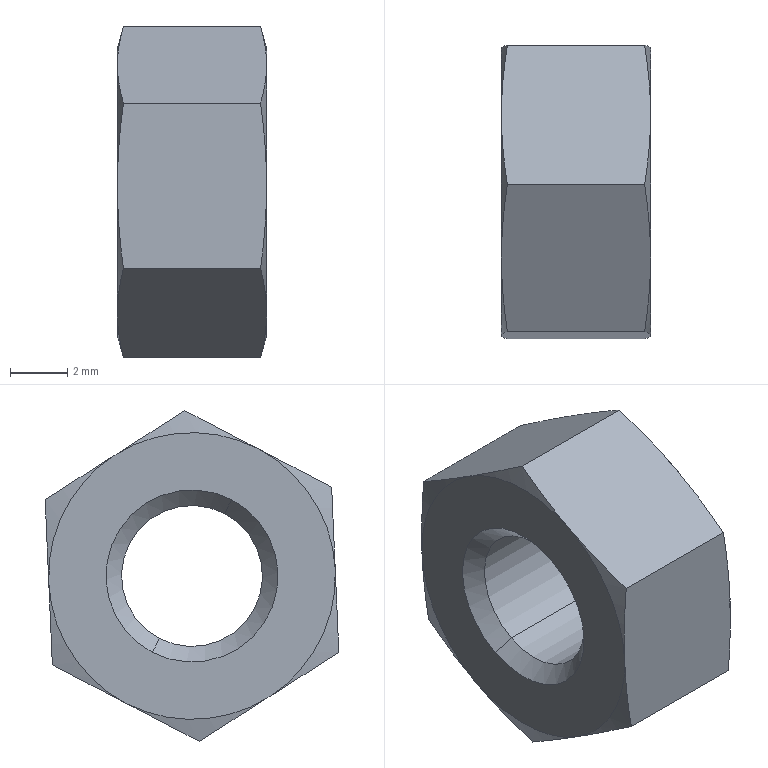Part | NX | features 2 2 | 1 solid | 26 faces | box 5.2 x 10.241 x 11.536 mm | volume 345.697 mm3 | cone 16 | plane 8 | cylinder 2 | commonest cylinder face diameters 4.917 x2
STEP:
#1=CARTESIAN_POINT('',(-91.959,96.265,-644.397));
#2=VERTEX_POINT('',#1);
#3=CARTESIAN_POINT('',(-91.959,93.994,-640.036));
#4=VERTEX_POINT('',#3);
#5=CARTESIAN_POINT('',(-91.959,95.129,-642.216));
#6=DIRECTION('',(1.,0.,0.));
#7=DIRECTION('',(0.,-0.4619,0.8869));
#8=AXIS2_PLACEMENT_3D('',#5,#6,#7);
#9=CIRCLE('',#8,2.458);
#10=EDGE_CURVE('',#2,#4,#9,.T.);
#11=ORIENTED_EDGE('',*,*,#10,.F.);
#12=CARTESIAN_POINT('',(-87.842,96.265,-644.397));
#13=VERTEX_POINT('',#12);
#14=CARTESIAN_POINT('',(-89.9,96.265,-644.397));
#15=DIRECTION('',(1.,0.,0.));
#16=VECTOR('',#15,1000.);
#17=LINE('',#14,#16);
#18=EDGE_CURVE('',#2,#13,#17,.T.);
#19=ORIENTED_EDGE('',*,*,#18,.T.);
#20=CARTESIAN_POINT('',(-87.842,93.994,-640.036));
#21=VERTEX_POINT('',#20);
#22=CARTESIAN_POINT('',(-87.842,95.129,-642.216));
#23=DIRECTION('',(-1.,0.,0.));
#24=DIRECTION('',(0.,-0.4619,0.8869));
#25=AXIS2_PLACEMENT_3D('',#22,#23,#24);
#26=CIRCLE('',#25,2.458);
#27=EDGE_CURVE('',#21,#13,#26,.T.);
#28=ORIENTED_EDGE('',*,*,#27,.F.);
#29=CARTESIAN_POINT('',(-89.9,93.994,-640.036));
#30=DIRECTION('',(1.,0.,0.));
#31=VECTOR('',#30,1000.);
#32=LINE('',#29,#31);
#33=EDGE_CURVE('',#21,#4,#32,.F.);
#34=ORIENTED_EDGE('',*,*,#33,.T.);
#35=EDGE_LOOP('',(#11,#19,#28,#34));
#36=FACE_BOUND('',#35,.T.);
#37=CARTESIAN_POINT('',(-89.9,95.129,-642.216));
#38=DIRECTION('',(1.,0.,0.));
#39=DIRECTION('',(0.,0.4619,-0.8869));
#40=AXIS2_PLACEMENT_3D('',#37,#38,#39);
#41=CYLINDRICAL_SURFACE('',#40,2.458);
#42=ADVANCED_FACE('',(#36),#41,.F.);
#43=ORIENTED_EDGE('',*,*,#10,.T.);
#44=CARTESIAN_POINT('',(-92.5,93.744,-639.556));
#45=VERTEX_POINT('',#44);
#46=CARTESIAN_POINT('',(-92.5,93.744,-639.556));
#47=DIRECTION('',(-0.7071,-0.3266,0.6272));
#48=VECTOR('',#47,1000.);
#49=LINE('',#46,#48);
#50=EDGE_CURVE('',#45,#4,#49,.F.);
#51=ORIENTED_EDGE('',*,*,#50,.F.);
#52=CARTESIAN_POINT('',(-92.5,96.515,-644.877));
#53=VERTEX_POINT('',#52);
#54=CARTESIAN_POINT('',(-92.5,95.129,-642.216));
#55=DIRECTION('',(1.,0.,0.));
#56=DIRECTION('',(0.,0.4619,-0.8869));
#57=AXIS2_PLACEMENT_3D('',#54,#55,#56);
#58=CIRCLE('',#57,3.);
#59=EDGE_CURVE('',#53,#45,#58,.T.);
#60=ORIENTED_EDGE('',*,*,#59,.F.);
#61=CARTESIAN_POINT('',(-92.5,96.515,-644.877));
#62=DIRECTION('',(-0.7071,0.3266,-0.6272));
#63=VECTOR('',#62,1000.);
#64=LINE('',#61,#63);
#65=EDGE_CURVE('',#2,#53,#64,.T.);
#66=ORIENTED_EDGE('',*,*,#65,.F.);
#67=EDGE_LOOP('',(#43,#51,#60,#66));
#68=FACE_BOUND('',#67,.T.);
#69=CARTESIAN_POINT('',(-92.5,95.129,-642.216));
#70=DIRECTION('',(-1.,0.,0.));
#71=DIRECTION('',(0.,-0.4619,0.8869));
#72=AXIS2_PLACEMENT_3D('',#69,#70,#71);
#73=CONICAL_SURFACE('',#72,3.,0.7854);
#74=ADVANCED_FACE('',(#68),#73,.F.);
#75=ORIENTED_EDGE('',*,*,#27,.T.);
#76=CARTESIAN_POINT('',(-87.3,96.515,-644.877));
#77=VERTEX_POINT('',#76);
#78=CARTESIAN_POINT('',(-87.3,96.515,-644.877));
#79=DIRECTION('',(0.7071,0.3266,-0.6272));
#80=VECTOR('',#79,1000.);
#81=LINE('',#78,#80);
#82=EDGE_CURVE('',#77,#13,#81,.F.);
#83=ORIENTED_EDGE('',*,*,#82,.F.);
#84=CARTESIAN_POINT('',(-87.3,93.744,-639.556));
#85=VERTEX_POINT('',#84);
#86=CARTESIAN_POINT('',(-87.3,95.129,-642.216));
#87=DIRECTION('',(-1.,0.,0.));
#88=DIRECTION('',(0.,-0.4619,0.8869));
#89=AXIS2_PLACEMENT_3D('',#86,#87,#88);
#90=CIRCLE('',#89,3.);
#91=EDGE_CURVE('',#85,#77,#90,.T.);
#92=ORIENTED_EDGE('',*,*,#91,.F.);
#93=CARTESIAN_POINT('',(-87.3,93.744,-639.556));
#94=DIRECTION('',(0.7071,-0.3266,0.6272));
#95=VECTOR('',#94,1000.);
#96=LINE('',#93,#95);
#97=EDGE_CURVE('',#21,#85,#96,.T.);
#98=ORIENTED_EDGE('',*,*,#97,.F.);
#99=EDGE_LOOP('',(#75,#83,#92,#98));
#100=FACE_BOUND('',#99,.T.);
#101=CARTESIAN_POINT('',(-87.3,95.129,-642.216));
#102=DIRECTION('',(1.,0.,0.));
#103=DIRECTION('',(0.,0.4619,-0.8869));
#104=AXIS2_PLACEMENT_3D('',#101,#102,#103);
#105=CONICAL_SURFACE('',#104,3.,0.7854);
#106=ADVANCED_FACE('',(#100),#105,.F.);
#107=ORIENTED_EDGE('',*,*,#18,.F.);
#108=CARTESIAN_POINT('',(-91.959,95.129,-642.216));
#109=DIRECTION('',(1.,0.,0.));
#110=DIRECTION('',(0.,-0.4619,0.8869));
#111=AXIS2_PLACEMENT_3D('',#108,#109,#110);
#112=CIRCLE('',#111,2.458);
#113=EDGE_CURVE('',#4,#2,#112,.T.);
#114=ORIENTED_EDGE('',*,*,#113,.F.);
#115=ORIENTED_EDGE('',*,*,#33,.F.);
#116=CARTESIAN_POINT('',(-87.842,95.129,-642.216));
#117=DIRECTION('',(-1.,0.,0.));
#118=DIRECTION('',(0.,-0.4619,0.8869));
#119=AXIS2_PLACEMENT_3D('',#116,#117,#118);
#120=CIRCLE('',#119,2.458);
#121=EDGE_CURVE('',#13,#21,#120,.T.);
#122=ORIENTED_EDGE('',*,*,#121,.F.);
#123=EDGE_LOOP('',(#107,#114,#115,#122));
#124=FACE_BOUND('',#123,.T.);
#125=CARTESIAN_POINT('',(-89.9,95.129,-642.216));
#126=DIRECTION('',(1.,0.,0.));
#127=DIRECTION('',(0.,0.4619,-0.8869));
#128=AXIS2_PLACEMENT_3D('',#125,#126,#127);
#129=CYLINDRICAL_SURFACE('',#128,2.458);
#130=ADVANCED_FACE('',(#124),#129,.F.);
#131=ORIENTED_EDGE('',*,*,#50,.T.);
#132=ORIENTED_EDGE('',*,*,#113,.T.);
#133=ORIENTED_EDGE('',*,*,#65,.T.);
#134=CARTESIAN_POINT('',(-92.5,95.129,-642.216));
#135=DIRECTION('',(1.,0.,0.));
#136=DIRECTION('',(0.,0.4619,-0.8869));
#137=AXIS2_PLACEMENT_3D('',#134,#135,#136);
#138=CIRCLE('',#137,3.);
#139=EDGE_CURVE('',#45,#53,#138,.T.);
#140=ORIENTED_EDGE('',*,*,#139,.F.);
#141=EDGE_LOOP('',(#131,#132,#133,#140));
#142=FACE_BOUND('',#141,.T.);
#143=CARTESIAN_POINT('',(-92.5,95.129,-642.216));
#144=DIRECTION('',(-1.,0.,0.));
#145=DIRECTION('',(0.,-0.4619,0.8869));
#146=AXIS2_PLACEMENT_3D('',#143,#144,#145);
#147=CONICAL_SURFACE('',#146,3.,0.7854);
#148=ADVANCED_FACE('',(#142),#147,.F.);
#149=ORIENTED_EDGE('',*,*,#82,.T.);
#150=ORIENTED_EDGE('',*,*,#121,.T.);
#151=ORIENTED_EDGE('',*,*,#97,.T.);
#152=CARTESIAN_POINT('',(-87.3,95.129,-642.216));
#153=DIRECTION('',(-1.,0.,0.));
#154=DIRECTION('',(0.,-0.4619,0.8869));
#155=AXIS2_PLACEMENT_3D('',#152,#153,#154);
#156=CIRCLE('',#155,3.);
#157=EDGE_CURVE('',#77,#85,#156,.T.);
#158=ORIENTED_EDGE('',*,*,#157,.F.);
#159=EDGE_LOOP('',(#149,#150,#151,#158));
#160=FACE_BOUND('',#159,.T.);
#161=CARTESIAN_POINT('',(-87.3,95.129,-642.216));
#162=DIRECTION('',(1.,0.,0.));
#163=DIRECTION('',(0.,0.4619,-0.8869));
#164=AXIS2_PLACEMENT_3D('',#161,#162,#163);
#165=CONICAL_SURFACE('',#164,3.,0.7854);
#166=ADVANCED_FACE('',(#160),#165,.F.);
#167=ORIENTED_EDGE('',*,*,#59,.T.);
#168=ORIENTED_EDGE('',*,*,#139,.T.);
#169=EDGE_LOOP('',(#167,#168));
#170=FACE_BOUND('',#169,.T.);
#171=CARTESIAN_POINT('',(-92.5,90.134,-641.999));
#172=VERTEX_POINT('',#171);
#173=CARTESIAN_POINT('',(-92.5,92.82,-637.782));
#174=VERTEX_POINT('',#173);
#175=CARTESIAN_POINT('',(-92.5,95.129,-642.216));
#176=DIRECTION('',(-1.,0.,0.));
#177=DIRECTION('',(0.,-0.4619,0.8869));
#178=AXIS2_PLACEMENT_3D('',#175,#176,#177);
#179=CIRCLE('',#178,5.);
#180=EDGE_CURVE('',#172,#174,#179,.T.);
#181=ORIENTED_EDGE('',*,*,#180,.T.);
#182=CARTESIAN_POINT('',(-92.5,97.815,-637.999));
#183=VERTEX_POINT('',#182);
#184=CARTESIAN_POINT('',(-92.5,95.129,-642.216));
#185=DIRECTION('',(-1.,0.,0.));
#186=DIRECTION('',(0.,-0.4619,0.8869));
#187=AXIS2_PLACEMENT_3D('',#184,#185,#186);
#188=CIRCLE('',#187,5.);
#189=EDGE_CURVE('',#174,#183,#188,.T.);
#190=ORIENTED_EDGE('',*,*,#189,.T.);
#191=CARTESIAN_POINT('',(-92.5,100.125,-642.434));
#192=VERTEX_POINT('',#191);
#193=CARTESIAN_POINT('',(-92.5,95.129,-642.216));
#194=DIRECTION('',(-1.,0.,0.));
#195=DIRECTION('',(0.,-0.4619,0.8869));
#196=AXIS2_PLACEMENT_3D('',#193,#194,#195);
#197=CIRCLE('',#196,5.);
#198=EDGE_CURVE('',#183,#192,#197,.T.);
#199=ORIENTED_EDGE('',*,*,#198,.T.);
#200=CARTESIAN_POINT('',(-92.5,97.439,-646.651));
#201=VERTEX_POINT('',#200);
#202=CARTESIAN_POINT('',(-92.5,95.129,-642.216));
#203=DIRECTION('',(-1.,0.,0.));
#204=DIRECTION('',(0.,-0.4619,0.8869));
#205=AXIS2_PLACEMENT_3D('',#202,#203,#204);
#206=CIRCLE('',#205,5.);
#207=EDGE_CURVE('',#192,#201,#206,.T.);
#208=ORIENTED_EDGE('',*,*,#207,.T.);
#209=CARTESIAN_POINT('',(-92.5,92.444,-646.434));
#210=VERTEX_POINT('',#209);
#211=CARTESIAN_POINT('',(-92.5,95.129,-642.216));
#212=DIRECTION('',(-1.,0.,0.));
#213=DIRECTION('',(0.,-0.4619,0.8869));
#214=AXIS2_PLACEMENT_3D('',#211,#212,#213);
#215=CIRCLE('',#214,5.);
#216=EDGE_CURVE('',#201,#210,#215,.T.);
#217=ORIENTED_EDGE('',*,*,#216,.T.);
#218=CARTESIAN_POINT('',(-92.5,95.129,-642.216));
#219=DIRECTION('',(-1.,0.,0.));
#220=DIRECTION('',(0.,-0.4619,0.8869));
#221=AXIS2_PLACEMENT_3D('',#218,#219,#220);
#222=CIRCLE('',#221,5.);
#223=EDGE_CURVE('',#210,#172,#222,.T.);
#224=ORIENTED_EDGE('',*,*,#223,.T.);
#225=EDGE_LOOP('',(#181,#190,#199,#208,#217,#224));
#226=FACE_BOUND('',#225,.T.);
#227=CARTESIAN_POINT('',(-92.5,97.347,-641.062));
#228=DIRECTION('',(-1.,0.,0.));
#229=DIRECTION('',(0.,-0.4619,0.8869));
#230=AXIS2_PLACEMENT_3D('',#227,#228,#229);
#231=PLANE('',#230);
#232=ADVANCED_FACE('',(#170,#226),#231,.T.);
#233=ORIENTED_EDGE('',*,*,#91,.T.);
#234=ORIENTED_EDGE('',*,*,#157,.T.);
#235=EDGE_LOOP('',(#233,#234));
#236=FACE_BOUND('',#235,.T.);
#237=CARTESIAN_POINT('',(-87.3,92.444,-646.434));
#238=VERTEX_POINT('',#237);
#239=CARTESIAN_POINT('',(-87.3,97.439,-646.651));
#240=VERTEX_POINT('',#239);
#241=CARTESIAN_POINT('',(-87.3,95.129,-642.216));
#242=DIRECTION('',(1.,0.,0.));
#243=DIRECTION('',(0.,0.4619,-0.8869));
#244=AXIS2_PLACEMENT_3D('',#241,#242,#243);
#245=CIRCLE('',#244,5.);
#246=EDGE_CURVE('',#238,#240,#245,.T.);
#247=ORIENTED_EDGE('',*,*,#246,.T.);
#248=CARTESIAN_POINT('',(-87.3,100.125,-642.434));
#249=VERTEX_POINT('',#248);
#250=CARTESIAN_POINT('',(-87.3,95.129,-642.216));
#251=DIRECTION('',(1.,0.,0.));
#252=DIRECTION('',(0.,0.4619,-0.8869));
#253=AXIS2_PLACEMENT_3D('',#250,#251,#252);
#254=CIRCLE('',#253,5.);
#255=EDGE_CURVE('',#240,#249,#254,.T.);
#256=ORIENTED_EDGE('',*,*,#255,.T.);
#257=CARTESIAN_POINT('',(-87.3,97.815,-637.999));
#258=VERTEX_POINT('',#257);
#259=CARTESIAN_POINT('',(-87.3,95.129,-642.216));
#260=DIRECTION('',(1.,0.,0.));
#261=DIRECTION('',(0.,0.4619,-0.8869));
#262=AXIS2_PLACEMENT_3D('',#259,#260,#261);
#263=CIRCLE('',#262,5.);
#264=EDGE_CURVE('',#249,#258,#263,.T.);
#265=ORIENTED_EDGE('',*,*,#264,.T.);
#266=CARTESIAN_POINT('',(-87.3,92.82,-637.782));
#267=VERTEX_POINT('',#266);
#268=CARTESIAN_POINT('',(-87.3,95.129,-642.216));
#269=DIRECTION('',(1.,0.,0.));
#270=DIRECTION('',(0.,0.4619,-0.8869));
#271=AXIS2_PLACEMENT_3D('',#268,#269,#270);
#272=CIRCLE('',#271,5.);
#273=EDGE_CURVE('',#258,#267,#272,.T.);
#274=ORIENTED_EDGE('',*,*,#273,.T.);
#275=CARTESIAN_POINT('',(-87.3,90.134,-641.999));
#276=VERTEX_POINT('',#275);
#277=CARTESIAN_POINT('',(-87.3,95.129,-642.216));
#278=DIRECTION('',(1.,0.,0.));
#279=DIRECTION('',(0.,0.4619,-0.8869));
#280=AXIS2_PLACEMENT_3D('',#277,#278,#279);
#281=CIRCLE('',#280,5.);
#282=EDGE_CURVE('',#267,#276,#281,.T.);
#283=ORIENTED_EDGE('',*,*,#282,.T.);
#284=CARTESIAN_POINT('',(-87.3,95.129,-642.216));
#285=DIRECTION('',(1.,0.,0.));
#286=DIRECTION('',(0.,0.4619,-0.8869));
#287=AXIS2_PLACEMENT_3D('',#284,#285,#286);
#288=CIRCLE('',#287,5.);
#289=EDGE_CURVE('',#276,#238,#288,.T.);
#290=ORIENTED_EDGE('',*,*,#289,.T.);
#291=EDGE_LOOP('',(#247,#256,#265,#274,#283,#290));
#292=FACE_BOUND('',#291,.T.);
#293=CARTESIAN_POINT('',(-87.3,97.347,-641.062));
#294=DIRECTION('',(1.,0.,0.));
#295=DIRECTION('',(0.,0.4619,-0.8869));
#296=AXIS2_PLACEMENT_3D('',#293,#294,#295);
#297=PLANE('',#296);
#298=ADVANCED_FACE('',(#236,#292),#297,.T.);
#299=CARTESIAN_POINT('',(-92.293,95.38,-636.448));
#300=VERTEX_POINT('',#299);
#301=CARTESIAN_POINT('',(-92.293,95.38,-636.448));
#302=CARTESIAN_POINT('',(-92.421,96.188,-636.963));
#303=CARTESIAN_POINT('',(-92.5,96.999,-637.479));
#304=CARTESIAN_POINT('',(-92.5,97.815,-637.999));
#305=B_SPLINE_CURVE_WITH_KNOTS('',3,(#301,#302,#303,#304),.UNSPECIFIED.,.F.,.F.,(4,4),(0.,0.002894),.UNSPECIFIED.);
#306=EDGE_CURVE('',#300,#183,#305,.T.);
#307=ORIENTED_EDGE('',*,*,#306,.T.);
#308=ORIENTED_EDGE('',*,*,#189,.F.);
#309=CARTESIAN_POINT('',(-92.5,92.82,-637.782));
#310=CARTESIAN_POINT('',(-92.5,93.678,-637.335));
#311=CARTESIAN_POINT('',(-92.421,94.531,-636.891));
#312=CARTESIAN_POINT('',(-92.293,95.38,-636.448));
#313=B_SPLINE_CURVE_WITH_KNOTS('',3,(#309,#310,#311,#312),.UNSPECIFIED.,.F.,.F.,(4,4),(0.,0.002894),.UNSPECIFIED.);
#314=EDGE_CURVE('',#174,#300,#313,.T.);
#315=ORIENTED_EDGE('',*,*,#314,.T.);
#316=EDGE_LOOP('',(#307,#308,#315));
#317=FACE_BOUND('',#316,.T.);
#318=CARTESIAN_POINT('',(-92.291,95.129,-642.216));
#319=DIRECTION('',(1.,0.,0.));
#320=DIRECTION('',(0.,0.4619,-0.8869));
#321=AXIS2_PLACEMENT_3D('',#318,#319,#320);
#322=CONICAL_SURFACE('',#321,5.778,1.309);
#323=ADVANCED_FACE('',(#317),#322,.T.);
#324=CARTESIAN_POINT('',(-92.293,90.26,-639.115));
#325=VERTEX_POINT('',#324);
#326=CARTESIAN_POINT('',(-92.293,90.26,-639.115));
#327=CARTESIAN_POINT('',(-92.421,91.109,-638.673));
#328=CARTESIAN_POINT('',(-92.5,91.962,-638.229));
#329=CARTESIAN_POINT('',(-92.5,92.82,-637.782));
#330=B_SPLINE_CURVE_WITH_KNOTS('',3,(#326,#327,#328,#329),.UNSPECIFIED.,.F.,.F.,(4,4),(0.,0.002894),.UNSPECIFIED.);
#331=EDGE_CURVE('',#325,#174,#330,.T.);
#332=ORIENTED_EDGE('',*,*,#331,.T.);
#333=ORIENTED_EDGE('',*,*,#180,.F.);
#334=CARTESIAN_POINT('',(-92.5,90.134,-641.999));
#335=CARTESIAN_POINT('',(-92.5,90.176,-641.033));
#336=CARTESIAN_POINT('',(-92.421,90.218,-640.072));
#337=CARTESIAN_POINT('',(-92.293,90.26,-639.115));
#338=B_SPLINE_CURVE_WITH_KNOTS('',3,(#334,#335,#336,#337),.UNSPECIFIED.,.F.,.F.,(4,4),(0.,0.002894),.UNSPECIFIED.);
#339=EDGE_CURVE('',#172,#325,#338,.T.);
#340=ORIENTED_EDGE('',*,*,#339,.T.);
#341=EDGE_LOOP('',(#332,#333,#340));
#342=FACE_BOUND('',#341,.T.);
#343=CARTESIAN_POINT('',(-92.291,95.129,-642.216));
#344=DIRECTION('',(1.,0.,0.));
#345=DIRECTION('',(0.,0.4619,-0.8869));
#346=AXIS2_PLACEMENT_3D('',#343,#344,#345);
#347=CONICAL_SURFACE('',#346,5.778,1.309);
#348=ADVANCED_FACE('',(#342),#347,.T.);
#349=CARTESIAN_POINT('',(-92.293,90.009,-644.883));
#350=VERTEX_POINT('',#349);
#351=CARTESIAN_POINT('',(-92.5,92.444,-646.434));
#352=CARTESIAN_POINT('',(-92.5,91.628,-645.914));
#353=CARTESIAN_POINT('',(-92.421,90.817,-645.398));
#354=CARTESIAN_POINT('',(-92.293,90.009,-644.883));
#355=B_SPLINE_CURVE_WITH_KNOTS('',3,(#351,#352,#353,#354),.UNSPECIFIED.,.F.,.F.,(4,4),(0.,0.002894),.UNSPECIFIED.);
#356=EDGE_CURVE('',#210,#350,#355,.T.);
#357=ORIENTED_EDGE('',*,*,#356,.T.);
#358=CARTESIAN_POINT('',(-92.293,90.009,-644.883));
#359=CARTESIAN_POINT('',(-92.421,90.05,-643.926));
#360=CARTESIAN_POINT('',(-92.5,90.092,-642.966));
#361=CARTESIAN_POINT('',(-92.5,90.134,-641.999));
#362=B_SPLINE_CURVE_WITH_KNOTS('',3,(#358,#359,#360,#361),.UNSPECIFIED.,.F.,.F.,(4,4),(0.,0.002894),.UNSPECIFIED.);
#363=EDGE_CURVE('',#350,#172,#362,.T.);
#364=ORIENTED_EDGE('',*,*,#363,.T.);
#365=ORIENTED_EDGE('',*,*,#223,.F.);
#366=EDGE_LOOP('',(#357,#364,#365));
#367=FACE_BOUND('',#366,.T.);
#368=CARTESIAN_POINT('',(-92.291,95.129,-642.216));
#369=DIRECTION('',(1.,0.,0.));
#370=DIRECTION('',(0.,0.4619,-0.8869));
#371=AXIS2_PLACEMENT_3D('',#368,#369,#370);
#372=CONICAL_SURFACE('',#371,5.778,1.309);
#373=ADVANCED_FACE('',(#367),#372,.T.);
#374=ORIENTED_EDGE('',*,*,#216,.F.);
#375=CARTESIAN_POINT('',(-92.293,94.879,-647.984));
#376=VERTEX_POINT('',#375);
#377=CARTESIAN_POINT('',(-92.5,97.439,-646.651));
#378=CARTESIAN_POINT('',(-92.5,96.581,-647.098));
#379=CARTESIAN_POINT('',(-92.421,95.728,-647.542));
#380=CARTESIAN_POINT('',(-92.293,94.879,-647.984));
#381=B_SPLINE_CURVE_WITH_KNOTS('',3,(#377,#378,#379,#380),.UNSPECIFIED.,.F.,.F.,(4,4),(0.,0.002894),.UNSPECIFIED.);
#382=EDGE_CURVE('',#201,#376,#381,.T.);
#383=ORIENTED_EDGE('',*,*,#382,.T.);
#384=CARTESIAN_POINT('',(-92.293,94.879,-647.984));
#385=CARTESIAN_POINT('',(-92.421,94.071,-647.47));
#386=CARTESIAN_POINT('',(-92.5,93.259,-646.953));
#387=CARTESIAN_POINT('',(-92.5,92.444,-646.434));
#388=B_SPLINE_CURVE_WITH_KNOTS('',3,(#384,#385,#386,#387),.UNSPECIFIED.,.F.,.F.,(4,4),(0.,0.002894),.UNSPECIFIED.);
#389=EDGE_CURVE('',#376,#210,#388,.T.);
#390=ORIENTED_EDGE('',*,*,#389,.T.);
#391=EDGE_LOOP('',(#374,#383,#390));
#392=FACE_BOUND('',#391,.T.);
#393=CARTESIAN_POINT('',(-92.291,95.129,-642.216));
#394=DIRECTION('',(1.,0.,0.));
#395=DIRECTION('',(0.,0.4619,-0.8869));
#396=AXIS2_PLACEMENT_3D('',#393,#394,#395);
#397=CONICAL_SURFACE('',#396,5.778,1.309);
#398=ADVANCED_FACE('',(#392),#397,.T.);
#399=ORIENTED_EDGE('',*,*,#207,.F.);
#400=CARTESIAN_POINT('',(-92.293,99.999,-645.318));
#401=VERTEX_POINT('',#400);
#402=CARTESIAN_POINT('',(-92.5,100.125,-642.434));
#403=CARTESIAN_POINT('',(-92.5,100.083,-643.4));
#404=CARTESIAN_POINT('',(-92.421,100.041,-644.361));
#405=CARTESIAN_POINT('',(-92.293,99.999,-645.318));
#406=B_SPLINE_CURVE_WITH_KNOTS('',3,(#402,#403,#404,#405),.UNSPECIFIED.,.F.,.F.,(4,4),(0.,0.002894),.UNSPECIFIED.);
#407=EDGE_CURVE('',#192,#401,#406,.T.);
#408=ORIENTED_EDGE('',*,*,#407,.T.);
#409=CARTESIAN_POINT('',(-92.293,99.999,-645.318));
#410=CARTESIAN_POINT('',(-92.421,99.15,-645.76));
#411=CARTESIAN_POINT('',(-92.5,98.297,-646.204));
#412=CARTESIAN_POINT('',(-92.5,97.439,-646.651));
#413=B_SPLINE_CURVE_WITH_KNOTS('',3,(#409,#410,#411,#412),.UNSPECIFIED.,.F.,.F.,(4,4),(0.,0.002894),.UNSPECIFIED.);
#414=EDGE_CURVE('',#401,#201,#413,.T.);
#415=ORIENTED_EDGE('',*,*,#414,.T.);
#416=EDGE_LOOP('',(#399,#408,#415));
#417=FACE_BOUND('',#416,.T.);
#418=CARTESIAN_POINT('',(-92.291,95.129,-642.216));
#419=DIRECTION('',(1.,0.,0.));
#420=DIRECTION('',(0.,0.4619,-0.8869));
#421=AXIS2_PLACEMENT_3D('',#418,#419,#420);
#422=CONICAL_SURFACE('',#421,5.778,1.309);
#423=ADVANCED_FACE('',(#417),#422,.T.);
#424=ORIENTED_EDGE('',*,*,#198,.F.);
#425=CARTESIAN_POINT('',(-92.293,100.25,-639.55));
#426=VERTEX_POINT('',#425);
#427=CARTESIAN_POINT('',(-92.5,97.815,-637.999));
#428=CARTESIAN_POINT('',(-92.5,98.631,-638.519));
#429=CARTESIAN_POINT('',(-92.421,99.442,-639.035));
#430=CARTESIAN_POINT('',(-92.293,100.25,-639.55));
#431=B_SPLINE_CURVE_WITH_KNOTS('',3,(#427,#428,#429,#430),.UNSPECIFIED.,.F.,.F.,(4,4),(0.,0.002894),.UNSPECIFIED.);
#432=EDGE_CURVE('',#183,#426,#431,.T.);
#433=ORIENTED_EDGE('',*,*,#432,.T.);
#434=CARTESIAN_POINT('',(-92.293,100.25,-639.55));
#435=CARTESIAN_POINT('',(-92.421,100.208,-640.507));
#436=CARTESIAN_POINT('',(-92.5,100.167,-641.467));
#437=CARTESIAN_POINT('',(-92.5,100.125,-642.434));
#438=B_SPLINE_CURVE_WITH_KNOTS('',3,(#434,#435,#436,#437),.UNSPECIFIED.,.F.,.F.,(4,4),(0.,0.002894),.UNSPECIFIED.);
#439=EDGE_CURVE('',#426,#192,#438,.T.);
#440=ORIENTED_EDGE('',*,*,#439,.T.);
#441=EDGE_LOOP('',(#424,#433,#440));
#442=FACE_BOUND('',#441,.T.);
#443=CARTESIAN_POINT('',(-92.291,95.129,-642.216));
#444=DIRECTION('',(1.,0.,0.));
#445=DIRECTION('',(0.,0.4619,-0.8869));
#446=AXIS2_PLACEMENT_3D('',#443,#444,#445);
#447=CONICAL_SURFACE('',#446,5.778,1.309);
#448=ADVANCED_FACE('',(#442),#447,.T.);
#449=CARTESIAN_POINT('',(-87.507,99.999,-645.318));
#450=VERTEX_POINT('',#449);
#451=CARTESIAN_POINT('',(-87.507,99.999,-645.318));
#452=CARTESIAN_POINT('',(-87.379,100.041,-644.361));
#453=CARTESIAN_POINT('',(-87.3,100.083,-643.4));
#454=CARTESIAN_POINT('',(-87.3,100.125,-642.434));
#455=B_SPLINE_CURVE_WITH_KNOTS('',3,(#451,#452,#453,#454),.UNSPECIFIED.,.F.,.F.,(4,4),(0.,0.002894),.UNSPECIFIED.);
#456=EDGE_CURVE('',#450,#249,#455,.T.);
#457=ORIENTED_EDGE('',*,*,#456,.T.);
#458=ORIENTED_EDGE('',*,*,#255,.F.);
#459=CARTESIAN_POINT('',(-87.3,97.439,-646.651));
#460=CARTESIAN_POINT('',(-87.3,98.297,-646.204));
#461=CARTESIAN_POINT('',(-87.379,99.15,-645.76));
#462=CARTESIAN_POINT('',(-87.507,99.999,-645.318));
#463=B_SPLINE_CURVE_WITH_KNOTS('',3,(#459,#460,#461,#462),.UNSPECIFIED.,.F.,.F.,(4,4),(0.,0.002894),.UNSPECIFIED.);
#464=EDGE_CURVE('',#240,#450,#463,.T.);
#465=ORIENTED_EDGE('',*,*,#464,.T.);
#466=EDGE_LOOP('',(#457,#458,#465));
#467=FACE_BOUND('',#466,.T.);
#468=CARTESIAN_POINT('',(-87.509,95.129,-642.216));
#469=DIRECTION('',(-1.,0.,0.));
#470=DIRECTION('',(0.,-0.4619,0.8869));
#471=AXIS2_PLACEMENT_3D('',#468,#469,#470);
#472=CONICAL_SURFACE('',#471,5.778,1.309);
#473=ADVANCED_FACE('',(#467),#472,.T.);
#474=ORIENTED_EDGE('',*,*,#246,.F.);
#475=CARTESIAN_POINT('',(-87.507,94.879,-647.984));
#476=VERTEX_POINT('',#475);
#477=CARTESIAN_POINT('',(-87.3,92.444,-646.434));
#478=CARTESIAN_POINT('',(-87.3,93.259,-646.953));
#479=CARTESIAN_POINT('',(-87.379,94.071,-647.47));
#480=CARTESIAN_POINT('',(-87.507,94.879,-647.984));
#481=B_SPLINE_CURVE_WITH_KNOTS('',3,(#477,#478,#479,#480),.UNSPECIFIED.,.F.,.F.,(4,4),(0.,0.002894),.UNSPECIFIED.);
#482=EDGE_CURVE('',#238,#476,#481,.T.);
#483=ORIENTED_EDGE('',*,*,#482,.T.);
#484=CARTESIAN_POINT('',(-87.507,94.879,-647.984));
#485=CARTESIAN_POINT('',(-87.379,95.728,-647.542));
#486=CARTESIAN_POINT('',(-87.3,96.581,-647.098));
#487=CARTESIAN_POINT('',(-87.3,97.439,-646.651));
#488=B_SPLINE_CURVE_WITH_KNOTS('',3,(#484,#485,#486,#487),.UNSPECIFIED.,.F.,.F.,(4,4),(0.,0.002894),.UNSPECIFIED.);
#489=EDGE_CURVE('',#476,#240,#488,.T.);
#490=ORIENTED_EDGE('',*,*,#489,.T.);
#491=EDGE_LOOP('',(#474,#483,#490));
#492=FACE_BOUND('',#491,.T.);
#493=CARTESIAN_POINT('',(-87.509,95.129,-642.216));
#494=DIRECTION('',(-1.,0.,0.));
#495=DIRECTION('',(0.,-0.4619,0.8869));
#496=AXIS2_PLACEMENT_3D('',#493,#494,#495);
#497=CONICAL_SURFACE('',#496,5.778,1.309);
#498=ADVANCED_FACE('',(#492),#497,.T.);
#499=ORIENTED_EDGE('',*,*,#289,.F.);
#500=CARTESIAN_POINT('',(-87.507,90.009,-644.883));
#501=VERTEX_POINT('',#500);
#502=CARTESIAN_POINT('',(-87.3,90.134,-641.999));
#503=CARTESIAN_POINT('',(-87.3,90.092,-642.966));
#504=CARTESIAN_POINT('',(-87.379,90.05,-643.926));
#505=CARTESIAN_POINT('',(-87.507,90.009,-644.883));
#506=B_SPLINE_CURVE_WITH_KNOTS('',3,(#502,#503,#504,#505),.UNSPECIFIED.,.F.,.F.,(4,4),(0.,0.002894),.UNSPECIFIED.);
#507=EDGE_CURVE('',#276,#501,#506,.T.);
#508=ORIENTED_EDGE('',*,*,#507,.T.);
#509=CARTESIAN_POINT('',(-87.507,90.009,-644.883));
#510=CARTESIAN_POINT('',(-87.379,90.817,-645.398));
#511=CARTESIAN_POINT('',(-87.3,91.628,-645.914));
#512=CARTESIAN_POINT('',(-87.3,92.444,-646.434));
#513=B_SPLINE_CURVE_WITH_KNOTS('',3,(#509,#510,#511,#512),.UNSPECIFIED.,.F.,.F.,(4,4),(0.,0.002894),.UNSPECIFIED.);
#514=EDGE_CURVE('',#501,#238,#513,.T.);
#515=ORIENTED_EDGE('',*,*,#514,.T.);
#516=EDGE_LOOP('',(#499,#508,#515));
#517=FACE_BOUND('',#516,.T.);
#518=CARTESIAN_POINT('',(-87.509,95.129,-642.216));
#519=DIRECTION('',(-1.,0.,0.));
#520=DIRECTION('',(0.,-0.4619,0.8869));
#521=AXIS2_PLACEMENT_3D('',#518,#519,#520);
#522=CONICAL_SURFACE('',#521,5.778,1.309);
#523=ADVANCED_FACE('',(#517),#522,.T.);
#524=ORIENTED_EDGE('',*,*,#282,.F.);
#525=CARTESIAN_POINT('',(-87.507,90.26,-639.115));
#526=VERTEX_POINT('',#525);
#527=CARTESIAN_POINT('',(-87.3,92.82,-637.782));
#528=CARTESIAN_POINT('',(-87.3,91.962,-638.229));
#529=CARTESIAN_POINT('',(-87.379,91.109,-638.673));
#530=CARTESIAN_POINT('',(-87.507,90.26,-639.115));
#531=B_SPLINE_CURVE_WITH_KNOTS('',3,(#527,#528,#529,#530),.UNSPECIFIED.,.F.,.F.,(4,4),(0.,0.002894),.UNSPECIFIED.);
#532=EDGE_CURVE('',#267,#526,#531,.T.);
#533=ORIENTED_EDGE('',*,*,#532,.T.);
#534=CARTESIAN_POINT('',(-87.507,90.26,-639.115));
#535=CARTESIAN_POINT('',(-87.379,90.218,-640.072));
#536=CARTESIAN_POINT('',(-87.3,90.176,-641.033));
#537=CARTESIAN_POINT('',(-87.3,90.134,-641.999));
#538=B_SPLINE_CURVE_WITH_KNOTS('',3,(#534,#535,#536,#537),.UNSPECIFIED.,.F.,.F.,(4,4),(0.,0.002894),.UNSPECIFIED.);
#539=EDGE_CURVE('',#526,#276,#538,.T.);
#540=ORIENTED_EDGE('',*,*,#539,.T.);
#541=EDGE_LOOP('',(#524,#533,#540));
#542=FACE_BOUND('',#541,.T.);
#543=CARTESIAN_POINT('',(-87.509,95.129,-642.216));
#544=DIRECTION('',(-1.,0.,0.));
#545=DIRECTION('',(0.,-0.4619,0.8869));
#546=AXIS2_PLACEMENT_3D('',#543,#544,#545);
#547=CONICAL_SURFACE('',#546,5.778,1.309);
#548=ADVANCED_FACE('',(#542),#547,.T.);
#549=CARTESIAN_POINT('',(-87.507,95.38,-636.448));
#550=VERTEX_POINT('',#549);
#551=CARTESIAN_POINT('',(-87.507,95.38,-636.448));
#552=CARTESIAN_POINT('',(-87.379,94.531,-636.891));
#553=CARTESIAN_POINT('',(-87.3,93.678,-637.335));
#554=CARTESIAN_POINT('',(-87.3,92.82,-637.782));
#555=B_SPLINE_CURVE_WITH_KNOTS('',3,(#551,#552,#553,#554),.UNSPECIFIED.,.F.,.F.,(4,4),(0.,0.002894),.UNSPECIFIED.);
#556=EDGE_CURVE('',#550,#267,#555,.T.);
#557=ORIENTED_EDGE('',*,*,#556,.T.);
#558=ORIENTED_EDGE('',*,*,#273,.F.);
#559=CARTESIAN_POINT('',(-87.3,97.815,-637.999));
#560=CARTESIAN_POINT('',(-87.3,96.999,-637.479));
#561=CARTESIAN_POINT('',(-87.379,96.188,-636.963));
#562=CARTESIAN_POINT('',(-87.507,95.38,-636.448));
#563=B_SPLINE_CURVE_WITH_KNOTS('',3,(#559,#560,#561,#562),.UNSPECIFIED.,.F.,.F.,(4,4),(0.,0.002894),.UNSPECIFIED.);
#564=EDGE_CURVE('',#258,#550,#563,.T.);
#565=ORIENTED_EDGE('',*,*,#564,.T.);
#566=EDGE_LOOP('',(#557,#558,#565));
#567=FACE_BOUND('',#566,.T.);
#568=CARTESIAN_POINT('',(-87.509,95.129,-642.216));
#569=DIRECTION('',(-1.,0.,0.));
#570=DIRECTION('',(0.,-0.4619,0.8869));
#571=AXIS2_PLACEMENT_3D('',#568,#569,#570);
#572=CONICAL_SURFACE('',#571,5.778,1.309);
#573=ADVANCED_FACE('',(#567),#572,.T.);
#574=CARTESIAN_POINT('',(-87.507,100.25,-639.55));
#575=VERTEX_POINT('',#574);
#576=CARTESIAN_POINT('',(-87.3,100.125,-642.434));
#577=CARTESIAN_POINT('',(-87.3,100.167,-641.467));
#578=CARTESIAN_POINT('',(-87.379,100.208,-640.507));
#579=CARTESIAN_POINT('',(-87.507,100.25,-639.55));
#580=B_SPLINE_CURVE_WITH_KNOTS('',3,(#576,#577,#578,#579),.UNSPECIFIED.,.F.,.F.,(4,4),(0.,0.002894),.UNSPECIFIED.);
#581=EDGE_CURVE('',#249,#575,#580,.T.);
#582=ORIENTED_EDGE('',*,*,#581,.T.);
#583=CARTESIAN_POINT('',(-87.507,100.25,-639.55));
#584=CARTESIAN_POINT('',(-87.379,99.442,-639.035));
#585=CARTESIAN_POINT('',(-87.3,98.631,-638.519));
#586=CARTESIAN_POINT('',(-87.3,97.815,-637.999));
#587=B_SPLINE_CURVE_WITH_KNOTS('',3,(#583,#584,#585,#586),.UNSPECIFIED.,.F.,.F.,(4,4),(0.,0.002894),.UNSPECIFIED.);
#588=EDGE_CURVE('',#575,#258,#587,.T.);
#589=ORIENTED_EDGE('',*,*,#588,.T.);
#590=ORIENTED_EDGE('',*,*,#264,.F.);
#591=EDGE_LOOP('',(#582,#589,#590));
#592=FACE_BOUND('',#591,.T.);
#593=CARTESIAN_POINT('',(-87.509,95.129,-642.216));
#594=DIRECTION('',(-1.,0.,0.));
#595=DIRECTION('',(0.,-0.4619,0.8869));
#596=AXIS2_PLACEMENT_3D('',#593,#594,#595);
#597=CONICAL_SURFACE('',#596,5.778,1.309);
#598=ADVANCED_FACE('',(#592),#597,.T.);
#599=CARTESIAN_POINT('',(-84.7,95.38,-636.448));
#600=DIRECTION('',(-1.,0.,0.));
#601=VECTOR('',#600,1000.);
#602=LINE('',#599,#601);
#603=EDGE_CURVE('',#550,#300,#602,.T.);
#604=ORIENTED_EDGE('',*,*,#603,.F.);
#605=ORIENTED_EDGE('',*,*,#564,.F.);
#606=ORIENTED_EDGE('',*,*,#588,.F.);
#607=CARTESIAN_POINT('',(-84.7,100.25,-639.55));
#608=DIRECTION('',(1.,0.,0.));
#609=VECTOR('',#608,1000.);
#610=LINE('',#607,#609);
#611=EDGE_CURVE('',#426,#575,#610,.T.);
#612=ORIENTED_EDGE('',*,*,#611,.F.);
#613=ORIENTED_EDGE('',*,*,#432,.F.);
#614=ORIENTED_EDGE('',*,*,#306,.F.);
#615=EDGE_LOOP('',(#604,#605,#606,#612,#613,#614));
#616=FACE_BOUND('',#615,.T.);
#617=CARTESIAN_POINT('',(-84.7,95.38,-636.448));
#618=DIRECTION('',(0.,-0.5371,-0.8435));
#619=DIRECTION('',(0.,0.8435,-0.5371));
#620=AXIS2_PLACEMENT_3D('',#617,#618,#619);
#621=PLANE('',#620);
#622=ADVANCED_FACE('',(#616),#621,.F.);
#623=CARTESIAN_POINT('',(-84.7,90.26,-639.115));
#624=DIRECTION('',(-1.,0.,0.));
#625=VECTOR('',#624,1000.);
#626=LINE('',#623,#625);
#627=EDGE_CURVE('',#526,#325,#626,.T.);
#628=ORIENTED_EDGE('',*,*,#627,.F.);
#629=ORIENTED_EDGE('',*,*,#532,.F.);
#630=ORIENTED_EDGE('',*,*,#556,.F.);
#631=ORIENTED_EDGE('',*,*,#603,.T.);
#632=ORIENTED_EDGE('',*,*,#314,.F.);
#633=ORIENTED_EDGE('',*,*,#331,.F.);
#634=EDGE_LOOP('',(#628,#629,#630,#631,#632,#633));
#635=FACE_BOUND('',#634,.T.);
#636=CARTESIAN_POINT('',(-84.7,90.26,-639.115));
#637=DIRECTION('',(0.,0.4619,-0.8869));
#638=DIRECTION('',(-1.,0.,0.));
#639=AXIS2_PLACEMENT_3D('',#636,#637,#638);
#640=PLANE('',#639);
#641=ADVANCED_FACE('',(#635),#640,.F.);
#642=CARTESIAN_POINT('',(-84.7,90.009,-644.883));
#643=DIRECTION('',(-1.,0.,0.));
#644=VECTOR('',#643,1000.);
#645=LINE('',#642,#644);
#646=EDGE_CURVE('',#501,#350,#645,.T.);
#647=ORIENTED_EDGE('',*,*,#646,.F.);
#648=ORIENTED_EDGE('',*,*,#507,.F.);
#649=ORIENTED_EDGE('',*,*,#539,.F.);
#650=ORIENTED_EDGE('',*,*,#627,.T.);
#651=ORIENTED_EDGE('',*,*,#339,.F.);
#652=ORIENTED_EDGE('',*,*,#363,.F.);
#653=EDGE_LOOP('',(#647,#648,#649,#650,#651,#652));
#654=FACE_BOUND('',#653,.T.);
#655=CARTESIAN_POINT('',(-84.7,90.009,-644.883));
#656=DIRECTION('',(0.,0.9991,-0.04344));
#657=DIRECTION('',(0.,0.04344,0.9991));
#658=AXIS2_PLACEMENT_3D('',#655,#656,#657);
#659=PLANE('',#658);
#660=ADVANCED_FACE('',(#654),#659,.F.);
#661=ORIENTED_EDGE('',*,*,#389,.F.);
#662=CARTESIAN_POINT('',(-84.7,94.879,-647.984));
#663=DIRECTION('',(-1.,0.,0.));
#664=VECTOR('',#663,1000.);
#665=LINE('',#662,#664);
#666=EDGE_CURVE('',#476,#376,#665,.T.);
#667=ORIENTED_EDGE('',*,*,#666,.F.);
#668=ORIENTED_EDGE('',*,*,#482,.F.);
#669=ORIENTED_EDGE('',*,*,#514,.F.);
#670=ORIENTED_EDGE('',*,*,#646,.T.);
#671=ORIENTED_EDGE('',*,*,#356,.F.);
#672=EDGE_LOOP('',(#661,#667,#668,#669,#670,#671));
#673=FACE_BOUND('',#672,.T.);
#674=CARTESIAN_POINT('',(-84.7,94.879,-647.984));
#675=DIRECTION('',(0.,0.5371,0.8435));
#676=DIRECTION('',(0.,-0.8435,0.5371));
#677=AXIS2_PLACEMENT_3D('',#674,#675,#676);
#678=PLANE('',#677);
#679=ADVANCED_FACE('',(#673),#678,.F.);
#680=ORIENTED_EDGE('',*,*,#414,.F.);
#681=CARTESIAN_POINT('',(-84.7,99.999,-645.318));
#682=DIRECTION('',(-1.,0.,0.));
#683=VECTOR('',#682,1000.);
#684=LINE('',#681,#683);
#685=EDGE_CURVE('',#450,#401,#684,.T.);
#686=ORIENTED_EDGE('',*,*,#685,.F.);
#687=ORIENTED_EDGE('',*,*,#464,.F.);
#688=ORIENTED_EDGE('',*,*,#489,.F.);
#689=ORIENTED_EDGE('',*,*,#666,.T.);
#690=ORIENTED_EDGE('',*,*,#382,.F.);
#691=EDGE_LOOP('',(#680,#686,#687,#688,#689,#690));
#692=FACE_BOUND('',#691,.T.);
#693=CARTESIAN_POINT('',(-84.7,99.999,-645.318));
#694=DIRECTION('',(0.,-0.4619,0.8869));
#695=DIRECTION('',(1.,0.,0.));
#696=AXIS2_PLACEMENT_3D('',#693,#694,#695);
#697=PLANE('',#696);
#698=ADVANCED_FACE('',(#692),#697,.F.);
#699=ORIENTED_EDGE('',*,*,#439,.F.);
#700=ORIENTED_EDGE('',*,*,#611,.T.);
#701=ORIENTED_EDGE('',*,*,#581,.F.);
#702=ORIENTED_EDGE('',*,*,#456,.F.);
#703=ORIENTED_EDGE('',*,*,#685,.T.);
#704=ORIENTED_EDGE('',*,*,#407,.F.);
#705=EDGE_LOOP('',(#699,#700,#701,#702,#703,#704));
#706=FACE_BOUND('',#705,.T.);
#707=CARTESIAN_POINT('',(-84.7,100.25,-639.55));
#708=DIRECTION('',(0.,-0.9991,0.04344));
#709=DIRECTION('',(0.,-0.04344,-0.9991));
#710=AXIS2_PLACEMENT_3D('',#707,#708,#709);
#711=PLANE('',#710);
#712=ADVANCED_FACE('',(#706),#711,.F.);
#713=CLOSED_SHELL('',(#42,#74,#106,#130,#148,#166,#232,#298,#323,#348,#373,#398,#423,#448,#473,#498,#523,#548,#573,#598,#622,#641,#660,#679,#698,#712));
#714=MANIFOLD_SOLID_BREP('',#713);
#715=(LENGTH_UNIT()NAMED_UNIT(*)SI_UNIT(.MILLI.,.METRE.));
#716=UNCERTAINTY_MEASURE_WITH_UNIT(LENGTH_MEASURE(0.0508),#715,'','');
#717=(NAMED_UNIT(*)PLANE_ANGLE_UNIT()SI_UNIT($,.RADIAN.));
#718=(NAMED_UNIT(*)SI_UNIT($,.STERADIAN.)SOLID_ANGLE_UNIT());
#719=(GEOMETRIC_REPRESENTATION_CONTEXT(3)GLOBAL_UNCERTAINTY_ASSIGNED_CONTEXT((#716))GLOBAL_UNIT_ASSIGNED_CONTEXT((#715,#717,#718))REPRESENTATION_CONTEXT('',''));
#720=ADVANCED_BREP_SHAPE_REPRESENTATION('',(#714),#719);